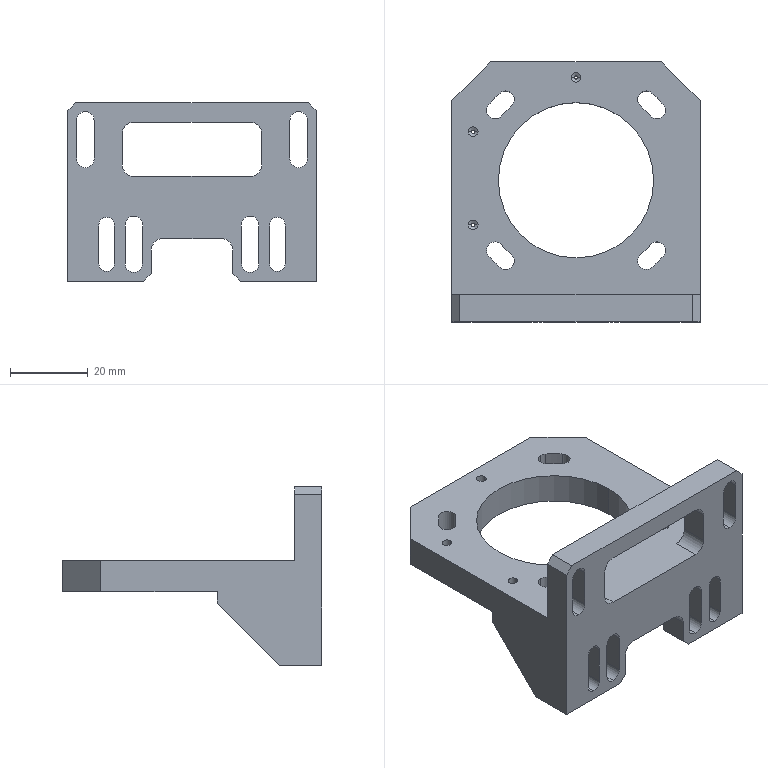NC program | NX | posted with a generic post | part box 64 x 67 x 46 mm
Lines 518 to 1940 of 30645:
(FLOOR_WALL_1_1 , TOOL : D10C)
N1028 T10 M6
N1030 G54
N1032 G17 G0 G90 X39.5 Y4.041 B0. C0. S2500 M3
N1034 G43 Z30. H10
N1036 Z0.9
N1038 G94 G1 Z-0.1 F1000.
N1040 X34. Y0.866
N1042 G3 X33.5 Y0. R1.
N1044 G1 Y-22. F2500.
N1046 X23.5 Y-32.
N1048 X-1.4
N1050 Y-22.9
N1052 X-21.4
N1054 Y22.9
N1056 X-1.4
N1058 Y32.
N1060 X23.5
N1062 X33.5 Y22.
N1064 Y0.
N1066 X26.5
N1068 Y-19.101
N1070 X20.601 Y-25.
N1072 X5.6
N1074 Y-22.9
N1076 G3 X-1.4 Y-15.9 R7.
N1078 G1 X-14.4
N1080 Y15.9
N1082 X-1.4
N1084 G3 X5.6 Y22.9 R7.
N1086 G1 Y25.
N1088 X20.601
N1090 X26.5 Y19.101
N1092 Y0.
N1094 X19.5
N1096 Y-16.201
N1098 X17.701 Y-18.
N1100 X11.714
N1102 G3 X-1.4 Y-8.9 R14.
N1104 G1 X-7.4
N1106 Y8.9
N1108 X-1.4
N1110 G3 X11.714 Y18. R14.
N1112 G1 X17.701
N1114 X19.5 Y16.201
N1116 Y0.
N1118 X12.5
N1120 Y-7.159
N1122 X14.365 Y-12.047
N1124 X12.5 Y-7.159
N1126 G3 X-0.4 Y-1.924 R21.
N1128 G1 Y1.924
N1130 G3 X12.5 Y7.159 R21.
N1132 G1 X14.365 Y12.047
N1134 X12.5 Y7.159
N1136 Y0.
N1138 G3 X13. Y-0.866 R1.
N1140 G1 Z0.9
N1142 G0 X39.5 Y4.041 Z0.8
N1144 G1 Z-0.2 F1000.
N1146 X34. Y0.866
N1148 G3 X33.5 Y0. R1.
N1150 G1 Y-22. F2500.
N1152 X23.5 Y-32.
N1154 X-1.4
N1156 Y-22.9
N1158 X-21.4
N1160 Y22.9
N1162 X-1.4
N1164 Y32.
N1166 X23.5
N1168 X33.5 Y22.
N1170 Y0.
N1172 X26.5
N1174 Y-19.101
N1176 X20.601 Y-25.
N1178 X5.6
N1180 Y-22.9
N1182 G3 X-1.4 Y-15.9 R7.
N1184 G1 X-14.4
N1186 Y15.9
N1188 X-1.4
N1190 G3 X5.6 Y22.9 R7.
N1192 G1 Y25.
N1194 X20.601
N1196 X26.5 Y19.101
N1198 Y0.
N1200 X19.5
N1202 Y-16.201
N1204 X17.701 Y-18.
N1206 X11.714
N1208 G3 X-1.4 Y-8.9 R14.
N1210 G1 X-7.4
N1212 Y8.9
N1214 X-1.4
N1216 G3 X11.714 Y18. R14.
N1218 G1 X17.701
N1220 X19.5 Y16.201
N1222 Y0.
N1224 X12.5
N1226 Y-7.159
N1228 X14.365 Y-12.047
N1230 X12.5 Y-7.159
N1232 G3 X-0.4 Y-1.924 R21.
N1234 G1 Y1.924
N1236 G3 X12.5 Y7.159 R21.
N1238 G1 X14.365 Y12.047
N1240 X12.5 Y7.159
N1242 Y0.
N1244 G3 X13. Y-0.866 R1.
N1246 G1 Z0.8
N1248 G0 X39.5 Y4.041 Z0.7
N1250 G1 Z-0.3 F1000.
N1252 X34. Y0.866
N1254 G3 X33.5 Y0. R1.
N1256 G1 Y-22. F2500.
N1258 X23.5 Y-32.
N1260 X-1.4
N1262 Y-22.9
N1264 X-21.4
N1266 Y22.9
N1268 X-1.4
N1270 Y32.
N1272 X23.5
N1274 X33.5 Y22.
N1276 Y0.
N1278 X26.5
N1280 Y-19.101
N1282 X20.601 Y-25.
N1284 X5.6
N1286 Y-22.9
N1288 G3 X-1.4 Y-15.9 R7.
N1290 G1 X-14.4
N1292 Y15.9
N1294 X-1.4
N1296 G3 X5.6 Y22.9 R7.
N1298 G1 Y25.
N1300 X20.601
N1302 X26.5 Y19.101
N1304 Y0.
N1306 X19.5
N1308 Y-16.201
N1310 X17.701 Y-18.
N1312 X11.714
N1314 G3 X-1.4 Y-8.9 R14.
N1316 G1 X-7.4
N1318 Y8.9
N1320 X-1.4
N1322 G3 X11.714 Y18. R14.
N1324 G1 X17.701
N1326 X19.5 Y16.201
N1328 Y0.
N1330 X12.5
N1332 Y-7.159
N1334 X14.365 Y-12.047
N1336 X12.5 Y-7.159
N1338 G3 X-0.4 Y-1.924 R21.
N1340 G1 Y1.924
N1342 G3 X12.5 Y7.159 R21.
N1344 G1 X14.365 Y12.047
N1346 X12.5 Y7.159
N1348 Y0.
N1350 G3 X13. Y-0.866 R1.
N1352 G1 Z0.7
N1354 G0 X39.5 Y4.041 Z0.6
N1356 G1 Z-0.4 F1000.
N1358 X34. Y0.866
N1360 G3 X33.5 Y0. R1.
N1362 G1 Y-22. F2500.
N1364 X23.5 Y-32.
N1366 X-1.4
N1368 Y-22.9
N1370 X-21.4
N1372 Y22.9
N1374 X-1.4
N1376 Y32.
N1378 X23.5
N1380 X33.5 Y22.
N1382 Y0.
N1384 X26.5
N1386 Y-19.101
N1388 X20.601 Y-25.
N1390 X5.6
N1392 Y-22.9
N1394 G3 X-1.4 Y-15.9 R7.
N1396 G1 X-14.4
N1398 Y15.9
N1400 X-1.4
N1402 G3 X5.6 Y22.9 R7.
N1404 G1 Y25.
N1406 X20.601
N1408 X26.5 Y19.101
N1410 Y0.
N1412 X19.5
N1414 Y-16.201
N1416 X17.701 Y-18.
N1418 X11.714
N1420 G3 X-1.4 Y-8.9 R14.
N1422 G1 X-7.4
N1424 Y8.9
N1426 X-1.4
N1428 G3 X11.714 Y18. R14.
N1430 G1 X17.701
N1432 X19.5 Y16.201
N1434 Y0.
N1436 X12.5
N1438 Y-7.159
N1440 X14.365 Y-12.047
N1442 X12.5 Y-7.159
N1444 G3 X-0.4 Y-1.924 R21.
N1446 G1 Y1.924
N1448 G3 X12.5 Y7.159 R21.
N1450 G1 X14.365 Y12.047
N1452 X12.5 Y7.159
N1454 Y0.
N1456 G3 X13. Y-0.866 R1.
N1458 G1 Z0.6
N1460 G0 X39.5 Y4.041 Z0.5
N1462 G1 Z-0.5 F1000.
N1464 X34. Y0.866
N1466 G3 X33.5 Y0. R1.
N1468 G1 Y-22. F2500.
N1470 X23.5 Y-32.
N1472 X-1.4
N1474 Y-22.9
N1476 X-21.4
N1478 Y22.9
N1480 X-1.4
N1482 Y32.
N1484 X23.5
N1486 X33.5 Y22.
N1488 Y0.
N1490 X26.5
N1492 Y-19.101
N1494 X20.601 Y-25.
N1496 X5.6
N1498 Y-22.9
N1500 G3 X-1.4 Y-15.9 R7.
N1502 G1 X-14.4
N1504 Y15.9
N1506 X-1.4
N1508 G3 X5.6 Y22.9 R7.
N1510 G1 Y25.
N1512 X20.601
N1514 X26.5 Y19.101
N1516 Y0.
N1518 X19.5
N1520 Y-16.201
N1522 X17.701 Y-18.
N1524 X11.714
N1526 G3 X-1.4 Y-8.9 R14.
N1528 G1 X-7.4
N1530 Y8.9
N1532 X-1.4
N1534 G3 X11.714 Y18. R14.
N1536 G1 X17.701
N1538 X19.5 Y16.201
N1540 Y0.
N1542 X12.5
N1544 Y-7.159
N1546 X14.365 Y-12.047
N1548 X12.5 Y-7.159
N1550 G3 X-0.4 Y-1.924 R21.
N1552 G1 Y1.924
N1554 G3 X12.5 Y7.159 R21.
N1556 G1 X14.365 Y12.047
N1558 X12.5 Y7.159
N1560 Y0.
N1562 G3 X13. Y-0.866 R1.
N1564 G1 Z0.5
N1566 G0 X39.5 Y4.041 Z0.4
N1568 G1 Z-0.6 F1000.
N1570 X34. Y0.866
N1572 G3 X33.5 Y0. R1.
N1574 G1 Y-22. F2500.
N1576 X23.5 Y-32.
N1578 X-1.4
N1580 Y-22.9
N1582 X-21.4
N1584 Y22.9
N1586 X-1.4
N1588 Y32.
N1590 X23.5
N1592 X33.5 Y22.
N1594 Y0.
N1596 X26.5
N1598 Y-19.101
N1600 X20.601 Y-25.
N1602 X5.6
N1604 Y-22.9
N1606 G3 X-1.4 Y-15.9 R7.
N1608 G1 X-14.4
N1610 Y15.9
N1612 X-1.4
N1614 G3 X5.6 Y22.9 R7.
N1616 G1 Y25.
N1618 X20.601
N1620 X26.5 Y19.101
N1622 Y0.
N1624 X19.5
N1626 Y-16.201
N1628 X17.701 Y-18.
N1630 X11.714
N1632 G3 X-1.4 Y-8.9 R14.
N1634 G1 X-7.4
N1636 Y8.9
N1638 X-1.4
N1640 G3 X11.714 Y18. R14.
N1642 G1 X17.701
N1644 X19.5 Y16.201
N1646 Y0.
N1648 X12.5
N1650 Y-7.159
N1652 X14.365 Y-12.047
N1654 X12.5 Y-7.159
N1656 G3 X-0.4 Y-1.924 R21.
N1658 G1 Y1.924
N1660 G3 X12.5 Y7.159 R21.
N1662 G1 X14.365 Y12.047
N1664 X12.5 Y7.159
N1666 Y0.
N1668 G3 X13. Y-0.866 R1.
N1670 G1 Z0.4
N1672 G0 X39.5 Y4.041 Z0.3
N1674 G1 Z-0.7 F1000.
N1676 X34. Y0.866
N1678 G3 X33.5 Y0. R1.
N1680 G1 Y-22. F2500.
N1682 X23.5 Y-32.
N1684 X-1.4
N1686 Y-22.9
N1688 X-21.4
N1690 Y22.9
N1692 X-1.4
N1694 Y32.
N1696 X23.5
N1698 X33.5 Y22.
N1700 Y0.
N1702 X26.5
N1704 Y-19.101
N1706 X20.601 Y-25.
N1708 X5.6
N1710 Y-22.9
N1712 G3 X-1.4 Y-15.9 R7.
N1714 G1 X-14.4
N1716 Y15.9
N1718 X-1.4
N1720 G3 X5.6 Y22.9 R7.
N1722 G1 Y25.
N1724 X20.601
N1726 X26.5 Y19.101
N1728 Y0.
N1730 X19.5
N1732 Y-16.201
N1734 X17.701 Y-18.
N1736 X11.714
N1738 G3 X-1.4 Y-8.9 R14.
N1740 G1 X-7.4
N1742 Y8.9
N1744 X-1.4
N1746 G3 X11.714 Y18. R14.
N1748 G1 X17.701
N1750 X19.5 Y16.201
N1752 Y0.
N1754 X12.5
N1756 Y-7.159
N1758 X14.365 Y-12.047
N1760 X12.5 Y-7.159
N1762 G3 X-0.4 Y-1.924 R21.
N1764 G1 Y1.924
N1766 G3 X12.5 Y7.159 R21.
N1768 G1 X14.365 Y12.047
N1770 X12.5 Y7.159
N1772 Y0.
N1774 G3 X13. Y-0.866 R1.
N1776 G1 Z0.3
N1778 G0 X39.5 Y4.041 Z0.2
N1780 G1 Z-0.8 F1000.
N1782 X34. Y0.866
N1784 G3 X33.5 Y0. R1.
N1786 G1 Y-22. F2500.
N1788 X23.5 Y-32.
N1790 X-1.4
N1792 Y-22.9
N1794 X-21.4
N1796 Y22.9
N1798 X-1.4
N1800 Y32.
N1802 X23.5
N1804 X33.5 Y22.
N1806 Y0.
N1808 X26.5
N1810 Y-19.101
N1812 X20.601 Y-25.
N1814 X5.6
N1816 Y-22.9
N1818 G3 X-1.4 Y-15.9 R7.
N1820 G1 X-14.4
N1822 Y15.9
N1824 X-1.4
N1826 G3 X5.6 Y22.9 R7.
N1828 G1 Y25.
N1830 X20.601
N1832 X26.5 Y19.101
N1834 Y0.
N1836 X19.5
N1838 Y-16.201
N1840 X17.701 Y-18.
N1842 X11.714
N1844 G3 X-1.4 Y-8.9 R14.
N1846 G1 X-7.4
N1848 Y8.9
N1850 X-1.4
N1852 G3 X11.714 Y18. R14.
N1854 G1 X17.701
N1856 X19.5 Y16.201
N1858 Y0.
N1860 X12.5
N1862 Y-7.159
N1864 X14.365 Y-12.047
N1866 X12.5 Y-7.159
N1868 G3 X-0.4 Y-1.924 R21.
N1870 G1 Y1.924
N1872 G3 X12.5 Y7.159 R21.
N1874 G1 X14.365 Y12.047
N1876 X12.5 Y7.159
N1878 Y0.
N1880 G3 X13. Y-0.866 R1.
N1882 G1 Z0.2
N1884 G0 X39.5 Y4.041 Z0.1
N1886 G1 Z-0.9 F1000.
N1888 X34. Y0.866
N1890 G3 X33.5 Y0. R1.
N1892 G1 Y-22. F2500.
N1894 X23.5 Y-32.
N1896 X-1.4
N1898 Y-22.9
N1900 X-21.4
N1902 Y22.9
N1904 X-1.4
N1906 Y32.
N1908 X23.5
N1910 X33.5 Y22.
N1912 Y0.
N1914 X26.5
N1916 Y-19.101
N1918 X20.601 Y-25.
N1920 X5.6
N1922 Y-22.9
N1924 G3 X-1.4 Y-15.9 R7.
N1926 G1 X-14.4
N1928 Y15.9
N1930 X-1.4
N1932 G3 X5.6 Y22.9 R7.
N1934 G1 Y25.
N1936 X20.601
N1938 X26.5 Y19.101
N1940 Y0.
N1942 X19.5
N1944 Y-16.201
N1946 X17.701 Y-18.
N1948 X11.714
N1950 G3 X-1.4 Y-8.9 R14.
N1952 G1 X-7.4
N1954 Y8.9
N1956 X-1.4
N1958 G3 X11.714 Y18. R14.
N1960 G1 X17.701
N1962 X19.5 Y16.201
N1964 Y0.
N1966 X12.5
N1968 Y-7.159
N1970 X14.365 Y-12.047
N1972 X12.5 Y-7.159
N1974 G3 X-0.4 Y-1.924 R21.
N1976 G1 Y1.924
N1978 G3 X12.5 Y7.159 R21.
N1980 G1 X14.365 Y12.047
N1982 X12.5 Y7.159
N1984 Y0.
N1986 G3 X13. Y-0.866 R1.
N1988 G1 Z0.1
N1990 G0 X39.5 Y4.041 Z0.
N1992 G1 Z-1. F1000.
N1994 X34. Y0.866
N1996 G3 X33.5 Y0. R1.
N1998 G1 Y-22. F2500.
N2000 X23.5 Y-32.
N2002 X-1.4
N2004 Y-22.9
N2006 X-21.4
N2008 Y22.9
N2010 X-1.4
N2012 Y32.
N2014 X23.5
N2016 X33.5 Y22.
N2018 Y0.
N2020 X26.5
N2022 Y-19.101
N2024 X20.601 Y-25.
N2026 X5.6
N2028 Y-22.9
N2030 G3 X-1.4 Y-15.9 R7.
N2032 G1 X-14.4
N2034 Y15.9
N2036 X-1.4
N2038 G3 X5.6 Y22.9 R7.
N2040 G1 Y25.
N2042 X20.601
N2044 X26.5 Y19.101
N2046 Y0.
N2048 X19.5
N2050 Y-16.201
N2052 X17.701 Y-18.
N2054 X11.714
N2056 G3 X-1.4 Y-8.9 R14.
N2058 G1 X-7.4
N2060 Y8.9
N2062 X-1.4
N2064 G3 X11.714 Y18. R14.
N2066 G1 X17.701
N2068 X19.5 Y16.201
N2070 Y0.
N2072 X12.5
N2074 Y-7.159
N2076 X14.365 Y-12.047
N2078 X12.5 Y-7.159
N2080 G3 X-0.4 Y-1.924 R21.
N2082 G1 Y1.924
N2084 G3 X12.5 Y7.159 R21.
N2086 G1 X14.365 Y12.047
N2088 X12.5 Y7.159
N2090 Y0.
N2092 G3 X13. Y-0.866 R1.
N2094 G1 Z0.
N2096 G0 X39.5 Y4.041 Z-0.1
N2098 G1 Z-1.1 F1000.
N2100 X34. Y0.866
N2102 G3 X33.5 Y0. R1.
N2104 G1 Y-22. F2500.
N2106 X23.5 Y-32.
N2108 X-1.4
N2110 Y-22.9
N2112 X-21.4
N2114 Y22.9
N2116 X-1.4
N2118 Y32.
N2120 X23.5
N2122 X33.5 Y22.
N2124 Y0.
N2126 X26.5
N2128 Y-19.101
N2130 X20.601 Y-25.
N2132 X5.6
N2134 Y-22.9
N2136 G3 X-1.4 Y-15.9 R7.
N2138 G1 X-14.4
N2140 Y15.9
N2142 X-1.4
N2144 G3 X5.6 Y22.9 R7.
N2146 G1 Y25.
N2148 X20.601
N2150 X26.5 Y19.101
N2152 Y0.
N2154 X19.5
N2156 Y-16.201
N2158 X17.701 Y-18.
N2160 X11.714
N2162 G3 X-1.4 Y-8.9 R14.
N2164 G1 X-7.4
N2166 Y8.9
N2168 X-1.4
N2170 G3 X11.714 Y18. R14.
N2172 G1 X17.701
N2174 X19.5 Y16.201
N2176 Y0.
N2178 X12.5
N2180 Y-7.159
N2182 X14.365 Y-12.047
N2184 X12.5 Y-7.159
N2186 G3 X-0.4 Y-1.924 R21.
N2188 G1 Y1.924
N2190 G3 X12.5 Y7.159 R21.
N2192 G1 X14.365 Y12.047
N2194 X12.5 Y7.159
N2196 Y0.
N2198 G3 X13. Y-0.866 R1.
N2200 G1 Z-0.1
N2202 G0 X39.5 Y4.041 Z-0.2
N2204 G1 Z-1.2 F1000.
N2206 X34. Y0.866
N2208 G3 X33.5 Y0. R1.
N2210 G1 Y-22. F2500.
N2212 X23.5 Y-32.
N2214 X-1.4
N2216 Y-22.9
N2218 X-21.4
N2220 Y22.9
N2222 X-1.4
N2224 Y32.
N2226 X23.5
N2228 X33.5 Y22.
N2230 Y0.
N2232 X26.5
N2234 Y-19.101
N2236 X20.601 Y-25.
N2238 X5.6
N2240 Y-22.9
N2242 G3 X-1.4 Y-15.9 R7.
N2244 G1 X-14.4
N2246 Y15.9
N2248 X-1.4
N2250 G3 X5.6 Y22.9 R7.
N2252 G1 Y25.
N2254 X20.601
N2256 X26.5 Y19.101
N2258 Y0.
N2260 X19.5
N2262 Y-16.201
N2264 X17.701 Y-18.
N2266 X11.714
N2268 G3 X-1.4 Y-8.9 R14.
N2270 G1 X-7.4
N2272 Y8.9
N2274 X-1.4
N2276 G3 X11.714 Y18. R14.
N2278 G1 X17.701
N2280 X19.5 Y16.201
N2282 Y0.
N2284 X12.5
N2286 Y-7.159
N2288 X14.365 Y-12.047
N2290 X12.5 Y-7.159
N2292 G3 X-0.4 Y-1.924 R21.
N2294 G1 Y1.924
N2296 G3 X12.5 Y7.159 R21.
N2298 G1 X14.365 Y12.047
N2300 X12.5 Y7.159
N2302 Y0.
N2304 G3 X13. Y-0.866 R1.
N2306 G1 Z-0.2
N2308 G0 X39.5 Y4.041 Z-0.3
N2310 G1 Z-1.3 F1000.
N2312 X34. Y0.866
N2314 G3 X33.5 Y0. R1.
N2316 G1 Y-22. F2500.
N2318 X23.5 Y-32.
N2320 X-1.4
N2322 Y-22.9
N2324 X-21.4
N2326 Y22.9
N2328 X-1.4
N2330 Y32.
N2332 X23.5
N2334 X33.5 Y22.
N2336 Y0.
N2338 X26.5
N2340 Y-19.101
N2342 X20.601 Y-25.
N2344 X5.6
N2346 Y-22.9
N2348 G3 X-1.4 Y-15.9 R7.
N2350 G1 X-14.4
N2352 Y15.9
N2354 X-1.4
N2356 G3 X5.6 Y22.9 R7.
N2358 G1 Y25.
N2360 X20.601
N2362 X26.5 Y19.101
N2364 Y0.
N2366 X19.5
N2368 Y-16.201
N2370 X17.701 Y-18.
N2372 X11.714
N2374 G3 X-1.4 Y-8.9 R14.
N2376 G1 X-7.4
N2378 Y8.9
N2380 X-1.4
N2382 G3 X11.714 Y18. R14.
N2384 G1 X17.701
N2386 X19.5 Y16.201
N2388 Y0.
N2390 X12.5
N2392 Y-7.159
N2394 X14.365 Y-12.047
N2396 X12.5 Y-7.159
N2398 G3 X-0.4 Y-1.924 R21.
N2400 G1 Y1.924
N2402 G3 X12.5 Y7.159 R21.
N2404 G1 X14.365 Y12.047
N2406 X12.5 Y7.159
N2408 Y0.
N2410 G3 X13. Y-0.866 R1.
N2412 G1 Z-0.3
N2414 G0 X39.5 Y4.041 Z-0.4
N2416 G1 Z-1.4 F1000.
N2418 X34. Y0.866
N2420 G3 X33.5 Y0. R1.
N2422 G1 Y-22. F2500.
N2424 X23.5 Y-32.
N2426 X-1.4
N2428 Y-22.9
N2430 X-21.4
N2432 Y22.9
N2434 X-1.4
N2436 Y32.
N2438 X23.5
N2440 X33.5 Y22.
N2442 Y0.
N2444 X26.5
N2446 Y-19.101
N2448 X20.601 Y-25.
N2450 X5.6
N2452 Y-22.9
N2454 G3 X-1.4 Y-15.9 R7.
N2456 G1 X-14.4
N2458 Y15.9
N2460 X-1.4
N2462 G3 X5.6 Y22.9 R7.
N2464 G1 Y25.
N2466 X20.601
N2468 X26.5 Y19.101
N2470 Y0.
N2472 X19.5
N2474 Y-16.201
N2476 X17.701 Y-18.
N2478 X11.714
N2480 G3 X-1.4 Y-8.9 R14.
N2482 G1 X-7.4
N2484 Y8.9
N2486 X-1.4
N2488 G3 X11.714 Y18. R14.
N2490 G1 X17.701
N2492 X19.5 Y16.201
N2494 Y0.
N2496 X12.5
N2498 Y-7.159
N2500 X14.365 Y-12.047
N2502 X12.5 Y-7.159
N2504 G3 X-0.4 Y-1.924 R21.
N2506 G1 Y1.924
N2508 G3 X12.5 Y7.159 R21.
N2510 G1 X14.365 Y12.047
N2512 X12.5 Y7.159
N2514 Y0.
N2516 G3 X13. Y-0.866 R1.
N2518 G1 Z-0.4
N2520 G0 X39.5 Y4.041 Z-0.5
N2522 G1 Z-1.5 F1000.
N2524 X34. Y0.866
N2526 G3 X33.5 Y0. R1.
N2528 G1 Y-22. F2500.
N2530 X23.5 Y-32.
N2532 X-1.4
N2534 Y-22.9
N2536 X-21.4
N2538 Y22.9
N2540 X-1.4
N2542 Y32.
N2544 X23.5
N2546 X33.5 Y22.
N2548 Y0.
N2550 X26.5
N2552 Y-19.101
N2554 X20.601 Y-25.
N2556 X5.6
N2558 Y-22.9
N2560 G3 X-1.4 Y-15.9 R7.
N2562 G1 X-14.4
N2564 Y15.9
N2566 X-1.4
N2568 G3 X5.6 Y22.9 R7.
N2570 G1 Y25.
N2572 X20.601
N2574 X26.5 Y19.101
N2576 Y0.
N2578 X19.5
N2580 Y-16.201
N2582 X17.701 Y-18.
N2584 X11.714
N2586 G3 X-1.4 Y-8.9 R14.
N2588 G1 X-7.4
N2590 Y8.9
N2592 X-1.4
N2594 G3 X11.714 Y18. R14.
N2596 G1 X17.701
N2598 X19.5 Y16.201
N2600 Y0.
N2602 X12.5
N2604 Y-7.159
N2606 X14.365 Y-12.047
N2608 X12.5 Y-7.159
N2610 G3 X-0.4 Y-1.924 R21.
N2612 G1 Y1.924
N2614 G3 X12.5 Y7.159 R21.
N2616 G1 X14.365 Y12.047
N2618 X12.5 Y7.159
N2620 Y0.
N2622 G3 X13. Y-0.866 R1.
N2624 G1 Z-0.5
N2626 G0 X39.5 Y4.041 Z-0.6
N2628 G1 Z-1.6 F1000.
N2630 X34. Y0.866
N2632 G3 X33.5 Y0. R1.
N2634 G1 Y-22. F2500.
N2636 X23.5 Y-32.
N2638 X-1.4
N2640 Y-22.9
N2642 X-21.4
N2644 Y22.9
N2646 X-1.4
N2648 Y32.
N2650 X23.5
N2652 X33.5 Y22.
N2654 Y0.
N2656 X26.5
N2658 Y-19.101
N2660 X20.601 Y-25.
N2662 X5.6
N2664 Y-22.9
N2666 G3 X-1.4 Y-15.9 R7.
N2668 G1 X-14.4
N2670 Y15.9
N2672 X-1.4
N2674 G3 X5.6 Y22.9 R7.
N2676 G1 Y25.
N2678 X20.601
N2680 X26.5 Y19.101
N2682 Y0.
N2684 X19.5
N2686 Y-16.201
N2688 X17.701 Y-18.
N2690 X11.714
N2692 G3 X-1.4 Y-8.9 R14.
N2694 G1 X-7.4
N2696 Y8.9
N2698 X-1.4
N2700 G3 X11.714 Y18. R14.
N2702 G1 X17.701
N2704 X19.5 Y16.201
N2706 Y0.
N2708 X12.5
N2710 Y-7.159
N2712 X14.365 Y-12.047
N2714 X12.5 Y-7.159
N2716 G3 X-0.4 Y-1.924 R21.
N2718 G1 Y1.924
N2720 G3 X12.5 Y7.159 R21.
N2722 G1 X14.365 Y12.047
N2724 X12.5 Y7.159
N2726 Y0.
N2728 G3 X13. Y-0.866 R1.
N2730 G1 Z-0.6
N2732 G0 X39.5 Y4.041 Z-0.7
N2734 G1 Z-1.7 F1000.
N2736 X34. Y0.866
N2738 G3 X33.5 Y0. R1.
N2740 G1 Y-22. F2500.
N2742 X23.5 Y-32.
N2744 X-1.4
N2746 Y-22.9
N2748 X-21.4
N2750 Y22.9
N2752 X-1.4
N2754 Y32.
N2756 X23.5
N2758 X33.5 Y22.
N2760 Y0.
N2762 X26.5
N2764 Y-19.101
N2766 X20.601 Y-25.
N2768 X5.6
N2770 Y-22.9
N2772 G3 X-1.4 Y-15.9 R7.
N2774 G1 X-14.4
N2776 Y15.9
N2778 X-1.4
N2780 G3 X5.6 Y22.9 R7.
N2782 G1 Y25.
N2784 X20.601
N2786 X26.5 Y19.101
N2788 Y0.
N2790 X19.5
N2792 Y-16.201
N2794 X17.701 Y-18.
N2796 X11.714
N2798 G3 X-1.4 Y-8.9 R14.
N2800 G1 X-7.4
N2802 Y8.9
N2804 X-1.4
N2806 G3 X11.714 Y18. R14.
N2808 G1 X17.701
N2810 X19.5 Y16.201
N2812 Y0.
N2814 X12.5
N2816 Y-7.159
N2818 X14.365 Y-12.047
N2820 X12.5 Y-7.159
N2822 G3 X-0.4 Y-1.924 R21.
N2824 G1 Y1.924
N2826 G3 X12.5 Y7.159 R21.
N2828 G1 X14.365 Y12.047
N2830 X12.5 Y7.159
N2832 Y0.
N2834 G3 X13. Y-0.866 R1.
N2836 G1 Z-0.7
N2838 G0 X39.5 Y4.041 Z-0.8
N2840 G1 Z-1.8 F1000.
N2842 X34. Y0.866
N2844 G3 X33.5 Y0. R1.
N2846 G1 Y-22. F2500.
N2848 X23.5 Y-32.
N2850 X-1.4
N2852 Y-22.9
N2854 X-21.4
N2856 Y22.9
N2858 X-1.4
N2860 Y32.
N2862 X23.5
N2864 X33.5 Y22.
N2866 Y0.
N2868 X26.5
N2870 Y-19.101
N2872 X20.601 Y-25.
N2874 X5.6
N2876 Y-22.9
N2878 G3 X-1.4 Y-15.9 R7.
N2880 G1 X-14.4
N2882 Y15.9
N2884 X-1.4
N2886 G3 X5.6 Y22.9 R7.
N2888 G1 Y25.
N2890 X20.601
N2892 X26.5 Y19.101
N2894 Y0.
N2896 X19.5
N2898 Y-16.201
N2900 X17.701 Y-18.
N2902 X11.714
N2904 G3 X-1.4 Y-8.9 R14.
N2906 G1 X-7.4
N2908 Y8.9
N2910 X-1.4
N2912 G3 X11.714 Y18. R14.
N2914 G1 X17.701
N2916 X19.5 Y16.201
N2918 Y0.
N2920 X12.5
N2922 Y-7.159
N2924 X14.365 Y-12.047
N2926 X12.5 Y-7.159
N2928 G3 X-0.4 Y-1.924 R21.
N2930 G1 Y1.924
N2932 G3 X12.5 Y7.159 R21.
N2934 G1 X14.365 Y12.047
N2936 X12.5 Y7.159
N2938 Y0.
N2940 G3 X13. Y-0.866 R1.
N2942 G1 Z-0.8
N2944 G0 X39.5 Y4.041 Z-0.9
N2946 G1 Z-1.9 F1000.
N2948 X34. Y0.866
N2950 G3 X33.5 Y0. R1.
N2952 G1 Y-22. F2500.
N2954 X23.5 Y-32.
N2956 X-1.4
N2958 Y-22.9
N2960 X-21.4
N2962 Y22.9
N2964 X-1.4
N2966 Y32.
N2968 X23.5
N2970 X33.5 Y22.
N2972 Y0.
N2974 X26.5
N2976 Y-19.101
N2978 X20.601 Y-25.
N2980 X5.6
N2982 Y-22.9
N2984 G3 X-1.4 Y-15.9 R7.
N2986 G1 X-14.4
N2988 Y15.9
N2990 X-1.4
N2992 G3 X5.6 Y22.9 R7.
N2994 G1 Y25.
N2996 X20.601
N2998 X26.5 Y19.101
N3000 Y0.
N3002 X19.5
N3004 Y-16.201
N3006 X17.701 Y-18.
N3008 X11.714
N3010 G3 X-1.4 Y-8.9 R14.
N3012 G1 X-7.4
N3014 Y8.9
N3016 X-1.4
N3018 G3 X11.714 Y18. R14.
N3020 G1 X17.701
N3022 X19.5 Y16.201
N3024 Y0.
N3026 X12.5
N3028 Y-7.159
N3030 X14.365 Y-12.047
N3032 X12.5 Y-7.159
N3034 G3 X-0.4 Y-1.924 R21.
N3036 G1 Y1.924
N3038 G3 X12.5 Y7.159 R21.
N3040 G1 X14.365 Y12.047
N3042 X12.5 Y7.159
N3044 Y0.
N3046 G3 X13. Y-0.866 R1.
N3048 G1 Z-0.9
N3050 G0 X39.5 Y4.041 Z-1.
N3052 G1 Z-2. F1000.
N3054 X34. Y0.866
N3056 G3 X33.5 Y0. R1.
N3058 G1 Y-22. F2500.
N3060 X23.5 Y-32.
N3062 X-1.4
N3064 Y-22.9
N3066 X-21.4
N3068 Y22.9
N3070 X-1.4
N3072 Y32.
N3074 X23.5
N3076 X33.5 Y22.
N3078 Y0.
N3080 X26.5
N3082 Y-19.101
N3084 X20.601 Y-25.
N3086 X5.6
N3088 Y-22.9
N3090 G3 X-1.4 Y-15.9 R7.
N3092 G1 X-14.4
N3094 Y15.9
N3096 X-1.4
N3098 G3 X5.6 Y22.9 R7.
N3100 G1 Y25.
N3102 X20.601
N3104 X26.5 Y19.101
N3106 Y0.
N3108 X19.5
N3110 Y-16.201
N3112 X17.701 Y-18.
N3114 X11.714
N3116 G3 X-1.4 Y-8.9 R14.
N3118 G1 X-7.4
N3120 Y8.9
N3122 X-1.4
N3124 G3 X11.714 Y18. R14.
N3126 G1 X17.701
N3128 X19.5 Y16.201
N3130 Y0.
N3132 X12.5
N3134 Y-7.159
N3136 X14.365 Y-12.047
N3138 X12.5 Y-7.159
N3140 G3 X-0.4 Y-1.924 R21.
N3142 G1 Y1.924
N3144 G3 X12.5 Y7.159 R21.
N3146 G1 X14.365 Y12.047
N3148 X12.5 Y7.159
N3150 Y0.
N3152 G3 X13. Y-0.866 R1.
N3154 G1 Z-1.
N3156 G0 X39.5 Y4.041 Z-1.1
N3158 G1 Z-2.1 F1000.
N3160 X34. Y0.866
N3162 G3 X33.5 Y0. R1.
N3164 G1 Y-22. F2500.
N3166 X23.5 Y-32.
N3168 X-1.4
N3170 Y-22.9
N3172 X-21.4
N3174 Y22.9
N3176 X-1.4
N3178 Y32.
N3180 X23.5
N3182 X33.5 Y22.
N3184 Y0.
N3186 X26.5
N3188 Y-19.101
N3190 X20.601 Y-25.
N3192 X5.6
N3194 Y-22.9
N3196 G3 X-1.4 Y-15.9 R7.
N3198 G1 X-14.4
N3200 Y15.9
N3202 X-1.4
N3204 G3 X5.6 Y22.9 R7.
N3206 G1 Y25.
N3208 X20.601
N3210 X26.5 Y19.101
N3212 Y0.
N3214 X19.5
N3216 Y-16.201
N3218 X17.701 Y-18.
N3220 X11.714
N3222 G3 X-1.4 Y-8.9 R14.
N3224 G1 X-7.4
N3226 Y8.9
N3228 X-1.4
N3230 G3 X11.714 Y18. R14.
N3232 G1 X17.701
N3234 X19.5 Y16.201
N3236 Y0.
N3238 X12.5
N3240 Y-7.159
N3242 X14.365 Y-12.047
N3244 X12.5 Y-7.159
N3246 G3 X-0.4 Y-1.924 R21.
N3248 G1 Y1.924
N3250 G3 X12.5 Y7.159 R21.
N3252 G1 X14.365 Y12.047
N3254 X12.5 Y7.159
N3256 Y0.
N3258 G3 X13. Y-0.866 R1.
N3260 G1 Z-1.1
N3262 G0 X39.5 Y4.041 Z-1.2
N3264 G1 Z-2.2 F1000.
N3266 X34. Y0.866
N3268 G3 X33.5 Y0. R1.
N3270 G1 Y-22. F2500.
N3272 X23.5 Y-32.
N3274 X-1.4
N3276 Y-22.9
N3278 X-21.4
N3280 Y22.9
N3282 X-1.4
N3284 Y32.
N3286 X23.5
N3288 X33.5 Y22.
N3290 Y0.
N3292 X26.5
N3294 Y-19.101
N3296 X20.601 Y-25.
N3298 X5.6
N3300 Y-22.9
N3302 G3 X-1.4 Y-15.9 R7.
N3304 G1 X-14.4
N3306 Y15.9
N3308 X-1.4
N3310 G3 X5.6 Y22.9 R7.
N3312 G1 Y25.
N3314 X20.601
N3316 X26.5 Y19.101
N3318 Y0.
N3320 X19.5
N3322 Y-16.201
N3324 X17.701 Y-18.
N3326 X11.714
N3328 G3 X-1.4 Y-8.9 R14.
N3330 G1 X-7.4
N3332 Y8.9
N3334 X-1.4
N3336 G3 X11.714 Y18. R14.
N3338 G1 X17.701
N3340 X19.5 Y16.201
N3342 Y0.
N3344 X12.5
N3346 Y-7.159
N3348 X14.365 Y-12.047
N3350 X12.5 Y-7.159
N3352 G3 X-0.4 Y-1.924 R21.
N3354 G1 Y1.924
N3356 G3 X12.5 Y7.159 R21.
N3358 G1 X14.365 Y12.047
N3360 X12.5 Y7.159
N3362 Y0.
N3364 G3 X13. Y-0.866 R1.
N3366 G1 Z-1.2
N3368 G0 X39.5 Y4.041 Z-1.3
N3370 G1 Z-2.3 F1000.
N3372 X34. Y0.866
N3374 G3 X33.5 Y0. R1.
N3376 G1 Y-22. F2500.
N3378 X23.5 Y-32.
N3380 X-1.4
N3382 Y-22.9
N3384 X-21.4
N3386 Y22.9
N3388 X-1.4
N3390 Y32.
N3392 X23.5
N3394 X33.5 Y22.
N3396 Y0.
N3398 X26.5
N3400 Y-19.101
N3402 X20.601 Y-25.
N3404 X5.6
N3406 Y-22.9
N3408 G3 X-1.4 Y-15.9 R7.
N3410 G1 X-14.4
N3412 Y15.9
N3414 X-1.4
N3416 G3 X5.6 Y22.9 R7.
N3418 G1 Y25.
N3420 X20.601
N3422 X26.5 Y19.101
N3424 Y0.
N3426 X19.5
N3428 Y-16.201
N3430 X17.701 Y-18.
N3432 X11.714
N3434 G3 X-1.4 Y-8.9 R14.
N3436 G1 X-7.4
N3438 Y8.9
N3440 X-1.4
N3442 G3 X11.714 Y18. R14.
N3444 G1 X17.701
N3446 X19.5 Y16.201
N3448 Y0.
N3450 X12.5
N3452 Y-7.159
N3454 X14.365 Y-12.047
N3456 X12.5 Y-7.159
N3458 G3 X-0.4 Y-1.924 R21.
N3460 G1 Y1.924
N3462 G3 X12.5 Y7.159 R21.
N3464 G1 X14.365 Y12.047
N3466 X12.5 Y7.159
N3468 Y0.
N3470 G3 X13. Y-0.866 R1.
N3472 G1 Z-1.3
N3474 G0 X39.5 Y4.041 Z-1.4
N3476 G1 Z-2.4 F1000.
N3478 X34. Y0.866
N3480 G3 X33.5 Y0. R1.
N3482 G1 Y-22. F2500.
N3484 X23.5 Y-32.
N3486 X-1.4
N3488 Y-22.9
N3490 X-21.4
N3492 Y22.9
N3494 X-1.4
N3496 Y32.
N3498 X23.5
N3500 X33.5 Y22.
N3502 Y0.
N3504 X26.5
N3506 Y-19.101
N3508 X20.601 Y-25.
N3510 X5.6
N3512 Y-22.9
N3514 G3 X-1.4 Y-15.9 R7.
N3516 G1 X-14.4
N3518 Y15.9
N3520 X-1.4
N3522 G3 X5.6 Y22.9 R7.
N3524 G1 Y25.
N3526 X20.601
N3528 X26.5 Y19.101
N3530 Y0.
N3532 X19.5
N3534 Y-16.201
N3536 X17.701 Y-18.
N3538 X11.714
N3540 G3 X-1.4 Y-8.9 R14.
N3542 G1 X-7.4
N3544 Y8.9
N3546 X-1.4
N3548 G3 X11.714 Y18. R14.
N3550 G1 X17.701
N3552 X19.5 Y16.201
N3554 Y0.
N3556 X12.5
N3558 Y-7.159
N3560 X14.365 Y-12.047
N3562 X12.5 Y-7.159
N3564 G3 X-0.4 Y-1.924 R21.
N3566 G1 Y1.924
N3568 G3 X12.5 Y7.159 R21.
N3570 G1 X14.365 Y12.047
N3572 X12.5 Y7.159
N3574 Y0.
N3576 G3 X13. Y-0.866 R1.
N3578 G1 Z-1.4
N3580 G0 X39.5 Y4.041 Z-1.5
N3582 G1 Z-2.5 F1000.
N3584 X34. Y0.866
N3586 G3 X33.5 Y0. R1.
N3588 G1 Y-22. F2500.
N3590 X23.5 Y-32.
N3592 X-1.4
N3594 Y-22.9
N3596 X-21.4
N3598 Y22.9
N3600 X-1.4
N3602 Y32.
N3604 X23.5
N3606 X33.5 Y22.
N3608 Y0.
N3610 X26.5
N3612 Y-19.101
N3614 X20.601 Y-25.
N3616 X5.6
N3618 Y-22.9
N3620 G3 X-1.4 Y-15.9 R7.
N3622 G1 X-14.4
N3624 Y15.9
N3626 X-1.4
N3628 G3 X5.6 Y22.9 R7.
N3630 G1 Y25.
N3632 X20.601
N3634 X26.5 Y19.101
N3636 Y0.
N3638 X19.5
N3640 Y-16.201
N3642 X17.701 Y-18.
N3644 X11.714
N3646 G3 X-1.4 Y-8.9 R14.
N3648 G1 X-7.4
N3650 Y8.9
N3652 X-1.4
N3654 G3 X11.714 Y18. R14.
N3656 G1 X17.701
N3658 X19.5 Y16.201
N3660 Y0.
N3662 X12.5
N3664 Y-7.159
N3666 X14.365 Y-12.047
N3668 X12.5 Y-7.159
N3670 G3 X-0.4 Y-1.924 R21.
N3672 G1 Y1.924
N3674 G3 X12.5 Y7.159 R21.
N3676 G1 X14.365 Y12.047
N3678 X12.5 Y7.159
N3680 Y0.
N3682 G3 X13. Y-0.866 R1.
N3684 G1 Z-1.5
N3686 G0 X39.5 Y4.041 Z-1.6
N3688 G1 Z-2.6 F1000.
N3690 X34. Y0.866
N3692 G3 X33.5 Y0. R1.
N3694 G1 Y-22. F2500.
N3696 X23.5 Y-32.
N3698 X-1.4
N3700 Y-22.9
N3702 X-21.4
N3704 Y22.9
N3706 X-1.4
N3708 Y32.
N3710 X23.5
N3712 X33.5 Y22.
N3714 Y0.
N3716 X26.5
N3718 Y-19.101
N3720 X20.601 Y-25.
N3722 X5.6
N3724 Y-22.9
N3726 G3 X-1.4 Y-15.9 R7.
N3728 G1 X-14.4
N3730 Y15.9
N3732 X-1.4
N3734 G3 X5.6 Y22.9 R7.
N3736 G1 Y25.
N3738 X20.601
N3740 X26.5 Y19.101
N3742 Y0.
N3744 X19.5
N3746 Y-16.201
N3748 X17.701 Y-18.
N3750 X11.714
N3752 G3 X-1.4 Y-8.9 R14.
N3754 G1 X-7.4
N3756 Y8.9
N3758 X-1.4
N3760 G3 X11.714 Y18. R14.
N3762 G1 X17.701
N3764 X19.5 Y16.201
N3766 Y0.
N3768 X12.5
N3770 Y-7.159
N3772 X14.365 Y-12.047
N3774 X12.5 Y-7.159
N3776 G3 X-0.4 Y-1.924 R21.
N3778 G1 Y1.924
N3780 G3 X12.5 Y7.159 R21.
N3782 G1 X14.365 Y12.047
N3784 X12.5 Y7.159
N3786 Y0.
N3788 G3 X13. Y-0.866 R1.
N3790 G1 Z-1.6
N3792 G0 X39.5 Y4.041 Z-1.7
N3794 G1 Z-2.7 F1000.
N3796 X34. Y0.866
N3798 G3 X33.5 Y0. R1.
N3800 G1 Y-22. F2500.
N3802 X23.5 Y-32.
N3804 X-1.4
N3806 Y-22.9
N3808 X-21.4
N3810 Y22.9
N3812 X-1.4
N3814 Y32.
N3816 X23.5
N3818 X33.5 Y22.
N3820 Y0.
N3822 X26.5
N3824 Y-19.101
N3826 X20.601 Y-25.
N3828 X5.6
N3830 Y-22.9
N3832 G3 X-1.4 Y-15.9 R7.
N3834 G1 X-14.4
N3836 Y15.9
N3838 X-1.4
N3840 G3 X5.6 Y22.9 R7.
N3842 G1 Y25.
N3844 X20.601
N3846 X26.5 Y19.101
N3848 Y0.
N3850 X19.5
N3852 Y-16.201
N3854 X17.701 Y-18.
N3856 X11.714
N3858 G3 X-1.4 Y-8.9 R14.
N3860 G1 X-7.4
N3862 Y8.9
N3864 X-1.4
N3866 G3 X11.714 Y18. R14.